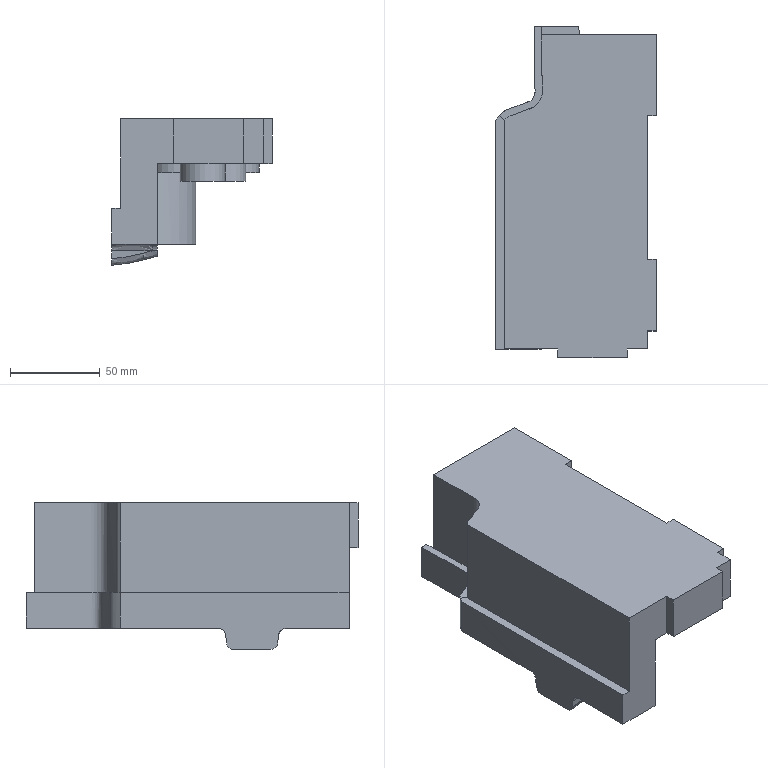Part | NX | features solid 2 | 1 solid | 54 faces | box 89.63 x 185 x 81.711 mm | volume 558064 mm3 | spline 26 | plane 24 | cylinder 4 | commonest cylinder face diameters 25 x2 30 x2